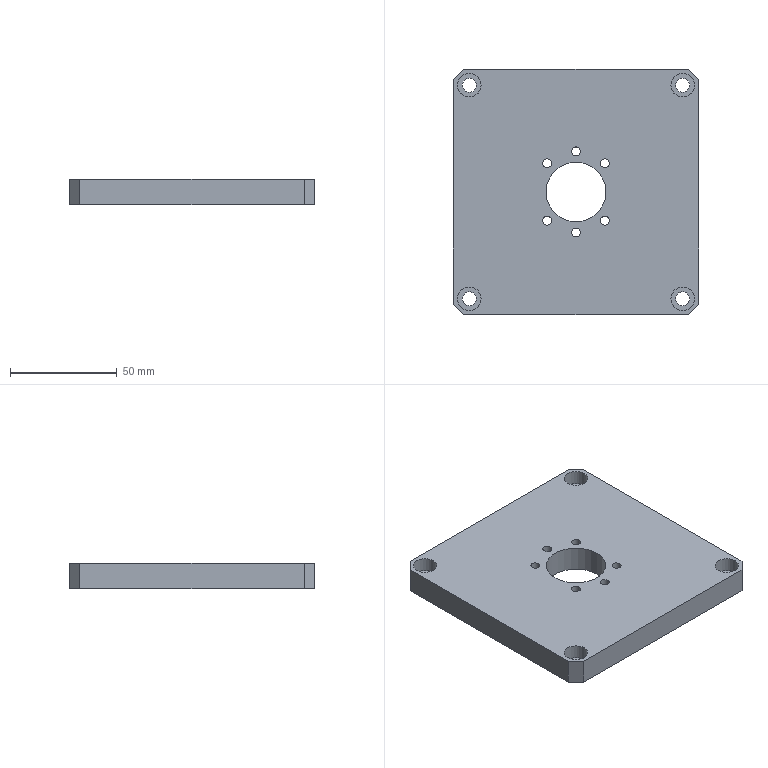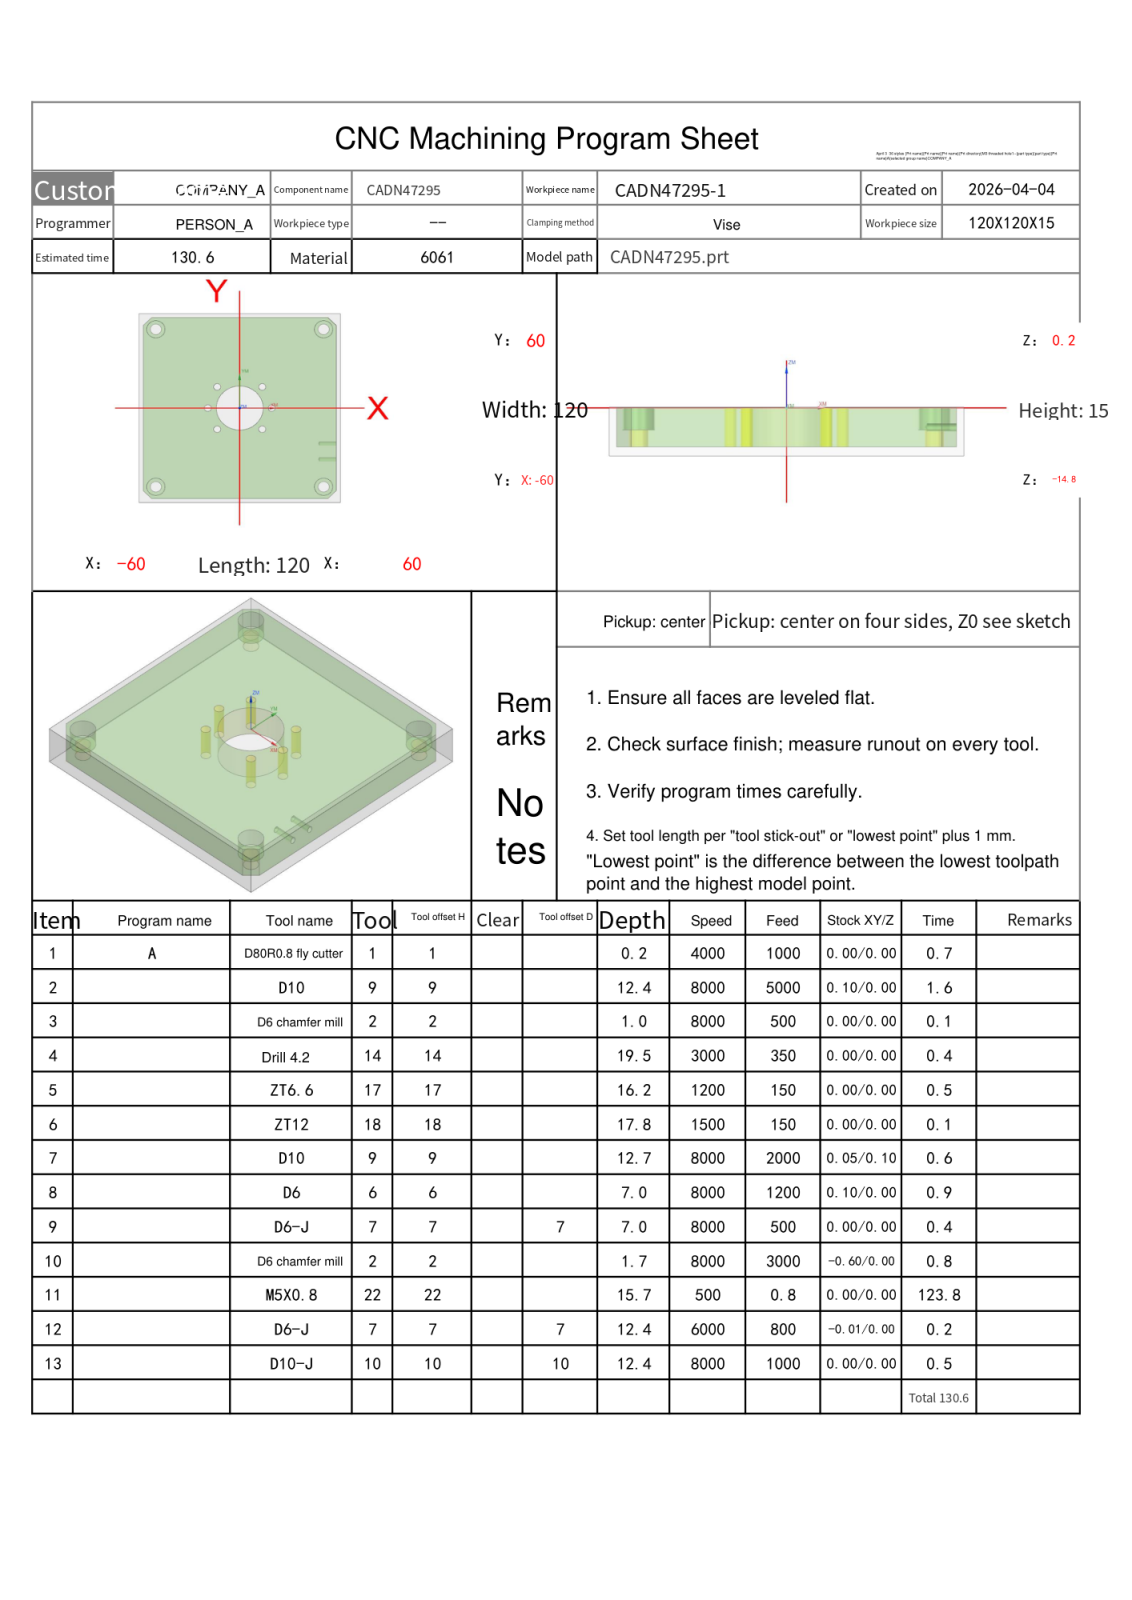NC program | NX | posted by the shop | part box 115 x 115 x 12 mm
Whole program:
%
O0001
(Machine time: 249.39 MIN)
(===Total Tool:10===)
(T1=D80R0.8 fly cutter D=80.  R=0.8  D-  H01 Z=0.    )
(T9=D10     D=10.  R=0.   D-  H09 Z=-12.5 )
(T2=D6 chamfer mill   D=6.   R=0.   D-  H02 Z=-1.5  )
(T14=drill 4.2  D=4.2  DR_a=118 D-  H14 Z=-19.26)
(T17=ZT6.6  D=6.6  DR_a=118 D-  H17 Z=-15.98)
(T18=ZT12   D=12.  DR_a=118 D-  H18 Z=-17.61)
(T6=D6      D=6.   R=0.   D-  H06 Z=-6.8  )
(T7=D6-J    D=6.   R=0.   D7  H07 Z=-12.2 )
(T22=M5X0.8 D=4.2  DR_a=180 D-  H22 Z=-15.5 )
(T10=D10-J  D=10.  R=0.   D10 H10 Z=-12.2 )
G80 G90 G17 G49 G40
G91 G28 Z0
M01
N1 T01 M06
(D80R0.8 fly cutter  D=80. R=0.8 H=01 ce=0.00 di=0.00)
G00 G90 G54 X48.75 Y102.5 M03 S4000
G43 H01 Z20.
M08
Z2.
G01 Z0.0 F1000.
Y97.5
Y-97.5
X0.0
Y97.5
X-48.75
Y-97.5
Y-102.5
Z2.
G00 Z20.
G91 G28 Z0.0
M05
M09
G91 G28 Z0.0
M01
N2 T09 M06
(D10  D=10. R=0. H=09 ce=0.10 di=0.00)
G00 G90 G54 X-62.6 Y0.0 M03 S8000
G43 H09 Z20.
M08
Z.5
G01 Y52.5 Z.413 F5000.
G02 X-61.106 Y56.106 Z.407 I5.1 J0.0
G01 X-56.106 Y61.106 Z.395
G02 X-52.5 Y62.6 Z.388 I3.606 J-3.606
G01 X52.5 Z.215
G02 X56.106 Y61.106 Z.208 I0.0 J-5.1
G01 X61.106 Y56.106 Z.197
G02 X62.6 Y52.5 Z.19 I-3.606 J-3.606
G01 Y-52.5 Z.016
G02 X61.106 Y-56.106 Z.01 I-5.1 J0.0
G01 X56.106 Y-61.106 Z-.002
G02 X52.5 Y-62.6 Z-.009 I-3.606 J3.606
G01 X-52.5 Z-.182
G02 X-56.106 Y-61.106 Z-.189 I0.0 J5.1
G01 X-61.106 Y-56.106 Z-.2
G02 X-62.6 Y-52.5 Z-.207 I3.606 J3.606
G01 Y52.5 Z-.381
G02 X-61.106 Y56.106 Z-.387 I5.1 J0.0
G01 X-56.106 Y61.106 Z-.399
G02 X-52.5 Y62.6 Z-.405 I3.606 J-3.606
G01 X52.5 Z-.579
G02 X56.106 Y61.106 Z-.586 I0.0 J-5.1
G01 X61.106 Y56.106 Z-.597
G02 X62.6 Y52.5 Z-.604 I-3.606 J-3.606
G01 Y-52.5 Z-.777
G02 X61.106 Y-56.106 Z-.784 I-5.1 J0.0
G01 X56.106 Y-61.106 Z-.796
G02 X52.5 Y-62.6 Z-.802 I-3.606 J3.606
G01 X-52.5 Z-.976
G02 X-56.106 Y-61.106 Z-.982 I0.0 J5.1
G01 X-61.106 Y-56.106 Z-.994
G02 X-62.6 Y-52.5 Z-1.001 I3.606 J3.606
G01 Y52.5 Z-1.174
G02 X-61.106 Y56.106 Z-1.181 I5.1 J0.0
G01 X-56.106 Y61.106 Z-1.193
G02 X-52.5 Y62.6 Z-1.199 I3.606 J-3.606
G01 X52.5 Z-1.373
G02 X56.106 Y61.106 Z-1.379 I0.0 J-5.1
G01 X61.106 Y56.106 Z-1.391
G02 X62.6 Y52.5 Z-1.398 I-3.606 J-3.606
G01 Y-52.5 Z-1.571
G02 X61.106 Y-56.106 Z-1.578 I-5.1 J0.0
G01 X56.106 Y-61.106 Z-1.589
G02 X52.5 Y-62.6 Z-1.596 I-3.606 J3.606
G01 X-52.5 Z-1.77
G02 X-56.106 Y-61.106 Z-1.776 I0.0 J5.1
G01 X-61.106 Y-56.106 Z-1.788
G02 X-62.6 Y-52.5 Z-1.794 I3.606 J3.606
G01 Y52.5 Z-1.968
G02 X-61.106 Y56.106 Z-1.975 I5.1 J0.0
G01 X-56.106 Y61.106 Z-1.986
G02 X-52.5 Y62.6 Z-1.993 I3.606 J-3.606
G01 X52.5 Z-2.166
G02 X56.106 Y61.106 Z-2.173 I0.0 J-5.1
G01 X61.106 Y56.106 Z-2.185
G02 X62.6 Y52.5 Z-2.191 I-3.606 J-3.606
G01 Y-52.5 Z-2.365
G02 X61.106 Y-56.106 Z-2.372 I-5.1 J0.0
G01 X56.106 Y-61.106 Z-2.383
G02 X52.5 Y-62.6 Z-2.39 I-3.606 J3.606
G01 X-52.5 Z-2.563
G02 X-56.106 Y-61.106 Z-2.57 I0.0 J5.1
G01 X-61.106 Y-56.106 Z-2.582
G02 X-62.6 Y-52.5 Z-2.588 I3.606 J3.606
G01 Y52.5 Z-2.762
G02 X-61.106 Y56.106 Z-2.768 I5.1 J0.0
G01 X-56.106 Y61.106 Z-2.78
G02 X-52.5 Y62.6 Z-2.787 I3.606 J-3.606
G01 X52.5 Z-2.96
G02 X56.106 Y61.106 Z-2.967 I0.0 J-5.1
G01 X61.106 Y56.106 Z-2.978
G02 X62.6 Y52.5 Z-2.985 I-3.606 J-3.606
G01 Y-52.5 Z-3.159
G02 X61.106 Y-56.106 Z-3.165 I-5.1 J0.0
G01 X56.106 Y-61.106 Z-3.177
G02 X52.5 Y-62.6 Z-3.184 I-3.606 J3.606
G01 X-52.5 Z-3.357
G02 X-56.106 Y-61.106 Z-3.364 I0.0 J5.1
G01 X-61.106 Y-56.106 Z-3.375
G02 X-62.6 Y-52.5 Z-3.382 I3.606 J3.606
G01 Y52.5 Z-3.556
G02 X-61.106 Y56.106 Z-3.562 I5.1 J0.0
G01 X-56.106 Y61.106 Z-3.574
G02 X-52.5 Y62.6 Z-3.58 I3.606 J-3.606
G01 X52.5 Z-3.754
G02 X56.106 Y61.106 Z-3.761 I0.0 J-5.1
G01 X61.106 Y56.106 Z-3.772
G02 X62.6 Y52.5 Z-3.779 I-3.606 J-3.606
G01 Y-52.5 Z-3.952
G02 X61.106 Y-56.106 Z-3.959 I-5.1 J0.0
G01 X56.106 Y-61.106 Z-3.971
G02 X52.5 Y-62.6 Z-3.977 I-3.606 J3.606
G01 X-52.5 Z-4.151
G02 X-56.106 Y-61.106 Z-4.157 I0.0 J5.1
G01 X-61.106 Y-56.106 Z-4.169
G02 X-62.6 Y-52.5 Z-4.176 I3.606 J3.606
G01 Y52.5 Z-4.349
G02 X-61.106 Y56.106 Z-4.356 I5.1 J0.0
G01 X-56.106 Y61.106 Z-4.368
G02 X-52.5 Y62.6 Z-4.374 I3.606 J-3.606
G01 X52.5 Z-4.548
G02 X56.106 Y61.106 Z-4.554 I0.0 J-5.1
G01 X61.106 Y56.106 Z-4.566
G02 X62.6 Y52.5 Z-4.573 I-3.606 J-3.606
G01 Y-52.5 Z-4.746
G02 X61.106 Y-56.106 Z-4.753 I-5.1 J0.0
G01 X56.106 Y-61.106 Z-4.764
G02 X52.5 Y-62.6 Z-4.771 I-3.606 J3.606
G01 X-52.5 Z-4.945
G02 X-56.106 Y-61.106 Z-4.951 I0.0 J5.1
G01 X-61.106 Y-56.106 Z-4.963
G02 X-62.6 Y-52.5 Z-4.969 I3.606 J3.606
G01 Y52.5 Z-5.143
G02 X-61.106 Y56.106 Z-5.15 I5.1 J0.0
G01 X-56.106 Y61.106 Z-5.161
G02 X-52.5 Y62.6 Z-5.168 I3.606 J-3.606
G01 X52.5 Z-5.341
G02 X56.106 Y61.106 Z-5.348 I0.0 J-5.1
G01 X61.106 Y56.106 Z-5.36
G02 X62.6 Y52.5 Z-5.366 I-3.606 J-3.606
G01 Y-52.5 Z-5.54
G02 X61.106 Y-56.106 Z-5.547 I-5.1 J0.0
G01 X56.106 Y-61.106 Z-5.558
G02 X52.5 Y-62.6 Z-5.565 I-3.606 J3.606
G01 X-52.5 Z-5.738
G02 X-56.106 Y-61.106 Z-5.745 I0.0 J5.1
G01 X-61.106 Y-56.106 Z-5.757
G02 X-62.6 Y-52.5 Z-5.763 I3.606 J3.606
G01 Y52.5 Z-5.937
G02 X-61.106 Y56.106 Z-5.943 I5.1 J0.0
G01 X-56.106 Y61.106 Z-5.955
G02 X-52.5 Y62.6 Z-5.962 I3.606 J-3.606
G01 X52.5 Z-6.135
G02 X56.106 Y61.106 Z-6.142 I0.0 J-5.1
G01 X61.106 Y56.106 Z-6.153
G02 X62.6 Y52.5 Z-6.16 I-3.606 J-3.606
G01 Y-52.5 Z-6.334
G02 X61.106 Y-56.106 Z-6.34 I-5.1 J0.0
G01 X56.106 Y-61.106 Z-6.352
G02 X52.5 Y-62.6 Z-6.359 I-3.606 J3.606
G01 X-52.5 Z-6.532
G02 X-56.106 Y-61.106 Z-6.539 I0.0 J5.1
G01 X-61.106 Y-56.106 Z-6.55
G02 X-62.6 Y-52.5 Z-6.557 I3.606 J3.606
G01 Y52.5 Z-6.731
G02 X-61.106 Y56.106 Z-6.737 I5.1 J0.0
G01 X-56.106 Y61.106 Z-6.749
G02 X-52.5 Y62.6 Z-6.755 I3.606 J-3.606
G01 X52.5 Z-6.929
G02 X56.106 Y61.106 Z-6.936 I0.0 J-5.1
G01 X61.106 Y56.106 Z-6.947
G02 X62.6 Y52.5 Z-6.954 I-3.606 J-3.606
G01 Y-52.5 Z-7.127
G02 X61.106 Y-56.106 Z-7.134 I-5.1 J0.0
G01 X56.106 Y-61.106 Z-7.146
G02 X52.5 Y-62.6 Z-7.152 I-3.606 J3.606
G01 X-52.5 Z-7.326
G02 X-56.106 Y-61.106 Z-7.332 I0.0 J5.1
G01 X-61.106 Y-56.106 Z-7.344
G02 X-62.6 Y-52.5 Z-7.351 I3.606 J3.606
G01 Y52.5 Z-7.524
G02 X-61.106 Y56.106 Z-7.531 I5.1 J0.0
G01 X-56.106 Y61.106 Z-7.543
G02 X-52.5 Y62.6 Z-7.549 I3.606 J-3.606
G01 X52.5 Z-7.723
G02 X56.106 Y61.106 Z-7.729 I0.0 J-5.1
G01 X61.106 Y56.106 Z-7.741
G02 X62.6 Y52.5 Z-7.748 I-3.606 J-3.606
G01 Y-52.5 Z-7.921
G02 X61.106 Y-56.106 Z-7.928 I-5.1 J0.0
G01 X56.106 Y-61.106 Z-7.939
G02 X52.5 Y-62.6 Z-7.946 I-3.606 J3.606
G01 X-52.5 Z-8.12
G02 X-56.106 Y-61.106 Z-8.126 I0.0 J5.1
G01 X-61.106 Y-56.106 Z-8.138
G02 X-62.6 Y-52.5 Z-8.144 I3.606 J3.606
G01 Y52.5 Z-8.318
G02 X-61.106 Y56.106 Z-8.325 I5.1 J0.0
G01 X-56.106 Y61.106 Z-8.336
G02 X-52.5 Y62.6 Z-8.343 I3.606 J-3.606
G01 X52.5 Z-8.516
G02 X56.106 Y61.106 Z-8.523 I0.0 J-5.1
G01 X61.106 Y56.106 Z-8.535
G02 X62.6 Y52.5 Z-8.541 I-3.606 J-3.606
G01 Y-52.5 Z-8.715
G02 X61.106 Y-56.106 Z-8.722 I-5.1 J0.0
G01 X56.106 Y-61.106 Z-8.733
G02 X52.5 Y-62.6 Z-8.74 I-3.606 J3.606
G01 X-52.5 Z-8.913
G02 X-56.106 Y-61.106 Z-8.92 I0.0 J5.1
G01 X-61.106 Y-56.106 Z-8.932
G02 X-62.6 Y-52.5 Z-8.938 I3.606 J3.606
G01 Y52.5 Z-9.112
G02 X-61.106 Y56.106 Z-9.118 I5.1 J0.0
G01 X-56.106 Y61.106 Z-9.13
G02 X-52.5 Y62.6 Z-9.137 I3.606 J-3.606
G01 X52.5 Z-9.31
G02 X56.106 Y61.106 Z-9.317 I0.0 J-5.1
G01 X61.106 Y56.106 Z-9.328
G02 X62.6 Y52.5 Z-9.335 I-3.606 J-3.606
G01 Y-52.5 Z-9.509
G02 X61.106 Y-56.106 Z-9.515 I-5.1 J0.0
G01 X56.106 Y-61.106 Z-9.527
G02 X52.5 Y-62.6 Z-9.534 I-3.606 J3.606
G01 X-52.5 Z-9.707
G02 X-56.106 Y-61.106 Z-9.714 I0.0 J5.1
G01 X-61.106 Y-56.106 Z-9.725
G02 X-62.6 Y-52.5 Z-9.732 I3.606 J3.606
G01 Y52.5 Z-9.906
G02 X-61.106 Y56.106 Z-9.912 I5.1 J0.0
G01 X-56.106 Y61.106 Z-9.924
G02 X-52.5 Y62.6 Z-9.93 I3.606 J-3.606
G01 X52.5 Z-10.104
G02 X56.106 Y61.106 Z-10.111 I0.0 J-5.1
G01 X61.106 Y56.106 Z-10.122
G02 X62.6 Y52.5 Z-10.129 I-3.606 J-3.606
G01 Y-52.5 Z-10.302
G02 X61.106 Y-56.106 Z-10.309 I-5.1 J0.0
G01 X56.106 Y-61.106 Z-10.321
G02 X52.5 Y-62.6 Z-10.327 I-3.606 J3.606
G01 X-52.5 Z-10.501
G02 X-56.106 Y-61.106 Z-10.507 I0.0 J5.1
G01 X-61.106 Y-56.106 Z-10.519
G02 X-62.6 Y-52.5 Z-10.526 I3.606 J3.606
G01 Y52.5 Z-10.699
G02 X-61.106 Y56.106 Z-10.706 I5.1 J0.0
G01 X-56.106 Y61.106 Z-10.718
G02 X-52.5 Y62.6 Z-10.724 I3.606 J-3.606
G01 X52.5 Z-10.898
G02 X56.106 Y61.106 Z-10.904 I0.0 J-5.1
G01 X61.106 Y56.106 Z-10.916
G02 X62.6 Y52.5 Z-10.923 I-3.606 J-3.606
G01 Y-52.5 Z-11.096
G02 X61.106 Y-56.106 Z-11.103 I-5.1 J0.0
G01 X56.106 Y-61.106 Z-11.114
G02 X52.5 Y-62.6 Z-11.121 I-3.606 J3.606
G01 X-52.5 Z-11.295
G02 X-56.106 Y-61.106 Z-11.301 I0.0 J5.1
G01 X-61.106 Y-56.106 Z-11.313
G02 X-62.6 Y-52.5 Z-11.319 I3.606 J3.606
G01 Y52.5 Z-11.493
G02 X-61.106 Y56.106 Z-11.5 I5.1 J0.0
G01 X-56.106 Y61.106 Z-11.511
G02 X-52.5 Y62.6 Z-11.518 I3.606 J-3.606
G01 X52.5 Z-11.691
G02 X56.106 Y61.106 Z-11.698 I0.0 J-5.1
G01 X61.106 Y56.106 Z-11.71
G02 X62.6 Y52.5 Z-11.716 I-3.606 J-3.606
G01 Y-52.5 Z-11.89
G02 X61.106 Y-56.106 Z-11.897 I-5.1 J0.0
G01 X56.106 Y-61.106 Z-11.908
G02 X52.5 Y-62.6 Z-11.915 I-3.606 J3.606
G01 X-52.5 Z-12.088
G02 X-56.106 Y-61.106 Z-12.095 I0.0 J5.1
G01 X-61.106 Y-56.106 Z-12.107
G02 X-62.6 Y-52.5 Z-12.113 I3.606 J3.606
G01 Y0.0 Z-12.2
Y52.5
G02 X-61.106 Y56.106 I5.1 J0.0
G01 X-56.106 Y61.106
G02 X-52.5 Y62.6 I3.606 J-3.606
G01 X52.5
G02 X56.106 Y61.106 I0.0 J-5.1
G01 X61.106 Y56.106
G02 X62.6 Y52.5 I-3.606 J-3.606
G01 Y-52.5
G02 X61.106 Y-56.106 I-5.1 J0.0
G01 X56.106 Y-61.106
G02 X52.5 Y-62.6 I-3.606 J3.606
G01 X-52.5
G02 X-56.106 Y-61.106 I0.0 J5.1
G01 X-61.106 Y-56.106
G02 X-62.6 Y-52.5 I3.606 J3.606
G01 Y0.0
Y.5
Z-11.2
G00 Z20.
G91 G28 Z0.0
M05
M09
G91 G28 Z0.0
M01
N3 T02 M06
(D6 chamfer mill  D=6. R=0. H=02 ce=0.00 di=0.00)
G00 G90 G54 X0.0 Y0.0 M03 S8000
G43 H02 Z20.
M08
G98 G82 X0.0 Y0.0 Z-.8 R1. F500.
G80
G00 Z20.
G00 G90 X50. Y50. M03 S8000
Z20.
G98 G81 X50. Y50. Z-.8 R1. F500.
X13.435 Y13.435
X19. Y0.0
X13.435 Y-13.435
X50. Y-50.
X-50.
X-13.435 Y-13.435
X-19. Y0.0
X-13.435 Y13.435
X-50. Y50.
G80
G00 Z20.
G91 G28 Z0.0
M05
M09
G91 G28 Z0.0
M01
N4 T14 M06
(drill 4.2 D=4.2 DR_a=118 H=14)
G00 G90 G54 X-13.435 Y-13.435 M03 S3000
G43 H14 Z20.
M08
G98 G83 X-13.435 Y-13.435 Z-19.262 R1. F350. Q3.
X-19. Y0.0
X-13.435 Y13.435
X13.435
X19. Y0.0
X13.435 Y-13.435
G80
G00 Z20.
G91 G28 Z0.0
M05
M09
G91 G28 Z0.0
M01
N5 T17 M06
(ZT6.6 D=6.6 DR_a=118 H=17)
G00 G90 G54 X-50. Y-50. M03 S1200
G43 H17 Z20.
M08
G98 G83 X-50. Y-50. Z-15.983 R1. F150. Q2.
Y50.
X50.
Y-50.
G80
G00 Z20.
G91 G28 Z0.0
M05
M09
G91 G28 Z0.0
M01
N6 T18 M06
(ZT12 D=12. DR_a=118 H=18)
G00 G90 G54 X0.0 Y0.0 M03 S800
G43 H18 Z20.
M08
G98 G83 X0.0 Y0.0 Z-17.605 R1. F150. Q3.
G80
G00 Z20.
G91 G28 Z0.0
M05
M09
G91 G28 Z0.0
M01
N7 T09 M06
(D10  D=10. R=0. H=09 ce=0.05 di=0.10)
G00 G90 G54 X-7.585 Y4.728 M03 S8000
G43 H09 Z20.
M08
Z1.
G01 X-7.949 Y4.177 Z.965 F2000.
X-8.623 Y2.506 Z.871
X-8.95 Y.733 Z.776
Y-.733 Z.7
X-8.623 Y-2.506 Z.605
X-7.949 Y-4.177 Z.511
X-6.955 Y-5.681 Z.416
X-5.681 Y-6.955 Z.322
X-4.177 Y-7.949 Z.227
X-2.506 Y-8.623 Z.133
X-.733 Y-8.95 Z.038
X0.0 Z0.0
G03 X8.95 Y0.0 Z-.149 I0.0 J8.95
X0.0 Y8.95 Z-.298 I-8.95 J0.0
X-8.95 Y0.0 Z-.446 I0.0 J-8.95
X0.0 Y-8.95 Z-.595 I8.95 J0.0
X8.95 Y0.0 Z-.744 I0.0 J8.95
X0.0 Y8.95 Z-.893 I-8.95 J0.0
X-8.95 Y0.0 Z-1.042 I0.0 J-8.95
X0.0 Y-8.95 Z-1.19 I8.95 J0.0
X8.95 Y0.0 Z-1.339 I0.0 J8.95
X0.0 Y8.95 Z-1.488 I-8.95 J0.0
X-8.95 Y0.0 Z-1.637 I0.0 J-8.95
X0.0 Y-8.95 Z-1.786 I8.95 J0.0
X8.95 Y0.0 Z-1.935 I0.0 J8.95
X0.0 Y8.95 Z-2.083 I-8.95 J0.0
X-8.95 Y0.0 Z-2.232 I0.0 J-8.95
X0.0 Y-8.95 Z-2.381 I8.95 J0.0
X8.95 Y0.0 Z-2.53 I0.0 J8.95
X0.0 Y8.95 Z-2.679 I-8.95 J0.0
X-8.95 Y0.0 Z-2.827 I0.0 J-8.95
X0.0 Y-8.95 Z-2.976 I8.95 J0.0
X8.95 Y0.0 Z-3.125 I0.0 J8.95
X0.0 Y8.95 Z-3.274 I-8.95 J0.0
X-8.95 Y0.0 Z-3.423 I0.0 J-8.95
X0.0 Y-8.95 Z-3.571 I8.95 J0.0
X8.95 Y0.0 Z-3.72 I0.0 J8.95
X0.0 Y8.95 Z-3.869 I-8.95 J0.0
X-8.95 Y0.0 Z-4.018 I0.0 J-8.95
X0.0 Y-8.95 Z-4.167 I8.95 J0.0
X8.95 Y0.0 Z-4.315 I0.0 J8.95
X0.0 Y8.95 Z-4.464 I-8.95 J0.0
X-8.95 Y0.0 Z-4.613 I0.0 J-8.95
X0.0 Y-8.95 Z-4.762 I8.95 J0.0
X8.95 Y0.0 Z-4.911 I0.0 J8.95
X0.0 Y8.95 Z-5.06 I-8.95 J0.0
X-8.95 Y0.0 Z-5.208 I0.0 J-8.95
X0.0 Y-8.95 Z-5.357 I8.95 J0.0
X8.95 Y0.0 Z-5.506 I0.0 J8.95
X0.0 Y8.95 Z-5.655 I-8.95 J0.0
X-8.95 Y0.0 Z-5.804 I0.0 J-8.95
X0.0 Y-8.95 Z-5.952 I8.95 J0.0
X8.95 Y0.0 Z-6.101 I0.0 J8.95
X0.0 Y8.95 Z-6.25 I-8.95 J0.0
X-8.95 Y0.0 Z-6.399 I0.0 J-8.95
X0.0 Y-8.95 Z-6.548 I8.95 J0.0
X8.95 Y0.0 Z-6.696 I0.0 J8.95
X0.0 Y8.95 Z-6.845 I-8.95 J0.0
X-8.95 Y0.0 Z-6.994 I0.0 J-8.95
X0.0 Y-8.95 Z-7.143 I8.95 J0.0
X8.95 Y0.0 Z-7.292 I0.0 J8.95
X0.0 Y8.95 Z-7.44 I-8.95 J0.0
X-8.95 Y0.0 Z-7.589 I0.0 J-8.95
X0.0 Y-8.95 Z-7.738 I8.95 J0.0
X8.95 Y0.0 Z-7.887 I0.0 J8.95
X0.0 Y8.95 Z-8.036 I-8.95 J0.0
X-8.95 Y0.0 Z-8.185 I0.0 J-8.95
X0.0 Y-8.95 Z-8.333 I8.95 J0.0
X8.95 Y0.0 Z-8.482 I0.0 J8.95
X0.0 Y8.95 Z-8.631 I-8.95 J0.0
X-8.95 Y0.0 Z-8.78 I0.0 J-8.95
X0.0 Y-8.95 Z-8.929 I8.95 J0.0
X8.95 Y0.0 Z-9.077 I0.0 J8.95
X0.0 Y8.95 Z-9.226 I-8.95 J0.0
X-8.95 Y0.0 Z-9.375 I0.0 J-8.95
X0.0 Y-8.95 Z-9.524 I8.95 J0.0
X8.95 Y0.0 Z-9.673 I0.0 J8.95
X0.0 Y8.95 Z-9.821 I-8.95 J0.0
X-8.95 Y0.0 Z-9.97 I0.0 J-8.95
X0.0 Y-8.95 Z-10.119 I8.95 J0.0
X8.95 Y0.0 Z-10.268 I0.0 J8.95
X0.0 Y8.95 Z-10.417 I-8.95 J0.0
X-8.95 Y0.0 Z-10.565 I0.0 J-8.95
X0.0 Y-8.95 Z-10.714 I8.95 J0.0
X8.95 Y0.0 Z-10.863 I0.0 J8.95
X0.0 Y8.95 Z-11.012 I-8.95 J0.0
X-8.95 Y0.0 Z-11.161 I0.0 J-8.95
X0.0 Y-8.95 Z-11.31 I8.95 J0.0
X8.95 Y0.0 Z-11.458 I0.0 J8.95
X0.0 Y8.95 Z-11.607 I-8.95 J0.0
X-8.95 Y0.0 Z-11.756 I0.0 J-8.95
X0.0 Y-8.95 Z-11.905 I8.95 J0.0
X8.95 Y0.0 Z-12.054 I0.0 J8.95
X0.0 Y8.95 Z-12.202 I-8.95 J0.0
X-8.95 Y0.0 Z-12.351 I0.0 J-8.95
X0.0 Y-8.95 Z-12.5 I8.95 J0.0
X8.95 Y0.0 I0.0 J8.95
X0.0 Y8.95 I-8.95 J0.0
X-8.95 Y0.0 I0.0 J-8.95
X0.0 Y-8.95 I8.95 J0.0
X.4 Y-8.941 I0.0 J8.95
G01 Z-11.5
G00 Z20.
G91 G28 Z0.0
M05
M09
G91 G28 Z0.0
M01
N8 T06 M06
(D6  D=6. R=0. H=06 ce=0.10 di=0.00)
G00 G90 G54 X-50. Y-50. M03 S8000
G43 H06 Z20.
M08
Z.5
G03 X-51.2 Y-51.2 I0.0 J-1.2 F1200.
X-50. Y-52.4 I1.2 J0.0
X-50. Y-52.4 Z0.0 I0.0 J2.4
X-50. Y-52.4 Z-.5 I0.0 J2.4
X-50. Y-52.4 Z-1. I0.0 J2.4
X-50. Y-52.4 Z-1.5 I0.0 J2.4
X-50. Y-52.4 Z-2. I0.0 J2.4
X-50. Y-52.4 Z-2.5 I0.0 J2.4
X-50. Y-52.4 Z-3. I0.0 J2.4
X-50. Y-52.4 Z-3.5 I0.0 J2.4
X-50. Y-52.4 Z-4. I0.0 J2.4
X-50. Y-52.4 Z-4.5 I0.0 J2.4
X-50. Y-52.4 Z-5. I0.0 J2.4
X-50. Y-52.4 Z-5.5 I0.0 J2.4
X-50. Y-52.4 Z-6. I0.0 J2.4
X-50. Y-52.4 Z-6.5 I0.0 J2.4
X-51.411 Y-48.058 Z-6.8 I0.0 J2.4
X-52.4 Y-50. I1.411 J-1.942
X-50. Y-52.4 I2.4 J0.0
X-47.6 Y-50. I0.0 J2.4
X-50. Y-47.6 I-2.4 J0.0
X-51.411 Y-48.058 I0.0 J-2.4
X-51.905 Y-49.029 I.705 J-.971
X-50.705 Y-50.229 I1.2 J0.0
X-50. Y-50. I0.0 J1.2
G00 Z20.
Y50.
Z.5
G03 X-51.2 Y48.8 I0.0 J-1.2
X-50. Y47.6 I1.2 J0.0
X-50. Y47.6 Z0.0 I0.0 J2.4
X-50. Y47.6 Z-.5 I0.0 J2.4
X-50. Y47.6 Z-1. I0.0 J2.4
X-50. Y47.6 Z-1.5 I0.0 J2.4
X-50. Y47.6 Z-2. I0.0 J2.4
X-50. Y47.6 Z-2.5 I0.0 J2.4
X-50. Y47.6 Z-3. I0.0 J2.4
X-50. Y47.6 Z-3.5 I0.0 J2.4
X-50. Y47.6 Z-4. I0.0 J2.4
X-50. Y47.6 Z-4.5 I0.0 J2.4
X-50. Y47.6 Z-5. I0.0 J2.4
X-50. Y47.6 Z-5.5 I0.0 J2.4
X-50. Y47.6 Z-6. I0.0 J2.4
X-50. Y47.6 Z-6.5 I0.0 J2.4
X-51.411 Y51.942 Z-6.8 I0.0 J2.4
X-52.4 Y50. I1.411 J-1.942
X-50. Y47.6 I2.4 J0.0
X-47.6 Y50. I0.0 J2.4
X-50. Y52.4 I-2.4 J0.0
X-51.411 Y51.942 I0.0 J-2.4
X-51.905 Y50.971 I.705 J-.971
X-50.705 Y49.771 I1.2 J0.0
X-50. Y50. I0.0 J1.2
G00 Z20.
X50.
Z.5
G03 X48.8 Y48.8 I0.0 J-1.2
X50. Y47.6 I1.2 J0.0
X50. Y47.6 Z0.0 I0.0 J2.4
X50. Y47.6 Z-.5 I0.0 J2.4
X50. Y47.6 Z-1. I0.0 J2.4
X50. Y47.6 Z-1.5 I0.0 J2.4
X50. Y47.6 Z-2. I0.0 J2.4
X50. Y47.6 Z-2.5 I0.0 J2.4
X50. Y47.6 Z-3. I0.0 J2.4
X50. Y47.6 Z-3.5 I0.0 J2.4
X50. Y47.6 Z-4. I0.0 J2.4
X50. Y47.6 Z-4.5 I0.0 J2.4
X50. Y47.6 Z-5. I0.0 J2.4
X50. Y47.6 Z-5.5 I0.0 J2.4
X50. Y47.6 Z-6. I0.0 J2.4
X50. Y47.6 Z-6.5 I0.0 J2.4
X48.589 Y51.942 Z-6.8 I0.0 J2.4
X47.6 Y50. I1.411 J-1.942
X50. Y47.6 I2.4 J0.0
X52.4 Y50. I0.0 J2.4
X50. Y52.4 I-2.4 J0.0
X48.589 Y51.942 I0.0 J-2.4
X48.095 Y50.971 I.705 J-.971
X49.295 Y49.771 I1.2 J0.0
X50. Y50. I0.0 J1.2
G00 Z20.
Y-50.
Z.5
G03 X48.8 Y-51.2 I0.0 J-1.2
X50. Y-52.4 I1.2 J0.0
X50. Y-52.4 Z0.0 I0.0 J2.4
X50. Y-52.4 Z-.5 I0.0 J2.4
X50. Y-52.4 Z-1. I0.0 J2.4
X50. Y-52.4 Z-1.5 I0.0 J2.4
X50. Y-52.4 Z-2. I0.0 J2.4
X50. Y-52.4 Z-2.5 I0.0 J2.4
X50. Y-52.4 Z-3. I0.0 J2.4
X50. Y-52.4 Z-3.5 I0.0 J2.4
X50. Y-52.4 Z-4. I0.0 J2.4
X50. Y-52.4 Z-4.5 I0.0 J2.4
X50. Y-52.4 Z-5. I0.0 J2.4
X50. Y-52.4 Z-5.5 I0.0 J2.4
X50. Y-52.4 Z-6. I0.0 J2.4
X50. Y-52.4 Z-6.5 I0.0 J2.4
X48.589 Y-48.058 Z-6.8 I0.0 J2.4
X47.6 Y-50. I1.411 J-1.942
X50. Y-52.4 I2.4 J0.0
X52.4 Y-50. I0.0 J2.4
X50. Y-47.6 I-2.4 J0.0
X48.589 Y-48.058 I0.0 J-2.4
X48.095 Y-49.029 I.705 J-.971
X49.295 Y-50.229 I1.2 J0.0
X50. Y-50. I0.0 J1.2
G00 Z20.
G91 G28 Z0.0
M05
M09
G91 G28 Z0.0
M01
N9 T07 M06
(D6-J  D=6. R=0. H=07 ce=0.00 di=0.00)
G00 G90 G54 X-50. Y-50. M03 S8000
G43 H07 Z20.
M08
Z0.0
G41 D07
G01 X-50.197 Y-50.032 F500.
G03 X-51.242 Y-51.258 I.197 J-1.226
X-50. Y-52.5 I1.242 J0.0
X-50. Y-52.5 Z-5. I0.0 J2.5
X-48.074 Y-48.406 Z-6.8 I0.0 J2.5
X-50. Y-47.5 I-1.926 J-1.594
X-52.5 Y-50. I0.0 J-2.5
X-50. Y-52.5 I2.5 J0.0
X-47.5 Y-50. I0.0 J2.5
X-48.074 Y-48.406 I-2.5 J0.0
X-49.031 Y-47.956 I-.957 J-.792
X-50.273 Y-49.198 I0.0 J-1.242
X-50.101 Y-49.828 I1.242 J0.0
G01 G40 X-50. Y-50.
G00 Z20.
Y50.
Z0.0
G41 D07
G01 X-50.197 Y49.968
G03 X-51.242 Y48.742 I.197 J-1.226
X-50. Y47.5 I1.242 J0.0
X-50. Y47.5 Z-5. I0.0 J2.5
X-48.074 Y51.594 Z-6.8 I0.0 J2.5
X-50. Y52.5 I-1.926 J-1.594
X-52.5 Y50. I0.0 J-2.5
X-50. Y47.5 I2.5 J0.0
X-47.5 Y50. I0.0 J2.5
X-48.074 Y51.594 I-2.5 J0.0
X-49.031 Y52.044 I-.957 J-.792
X-50.273 Y50.802 I0.0 J-1.242
X-50.101 Y50.172 I1.242 J0.0
G01 G40 X-50. Y50.
G00 Z20.
X50.
Z0.0
G41 D07
G01 X49.803 Y49.968
G03 X48.758 Y48.742 I.197 J-1.226
X50. Y47.5 I1.242 J0.0
X50. Y47.5 Z-5. I0.0 J2.5
X51.926 Y51.594 Z-6.8 I0.0 J2.5
X50. Y52.5 I-1.926 J-1.594
X47.5 Y50. I0.0 J-2.5
X50. Y47.5 I2.5 J0.0
X52.5 Y50. I0.0 J2.5
X51.926 Y51.594 I-2.5 J0.0
X50.969 Y52.044 I-.957 J-.792
X49.727 Y50.802 I0.0 J-1.242
X49.899 Y50.172 I1.242 J0.0
G01 G40 X50. Y50.
G00 Z20.
Y-50.
Z0.0
G41 D07
G01 X49.803 Y-50.032
G03 X48.758 Y-51.258 I.197 J-1.226
X50. Y-52.5 I1.242 J0.0
X50. Y-52.5 Z-5. I0.0 J2.5
X51.926 Y-48.406 Z-6.8 I0.0 J2.5
X50. Y-47.5 I-1.926 J-1.594
X47.5 Y-50. I0.0 J-2.5
X50. Y-52.5 I2.5 J0.0
X52.5 Y-50. I0.0 J2.5
X51.926 Y-48.406 I-2.5 J0.0
X50.969 Y-47.956 I-.957 J-.792
X49.727 Y-49.198 I0.0 J-1.242
X49.899 Y-49.828 I1.242 J0.0
G01 G40 X50. Y-50.
G00 Z20.
G91 G28 Z0.0
M05
M09
G91 G28 Z0.0
M01
N10 T02 M06
(D6 chamfer mill  D=6. R=0. H=02 ce=0.00 di=0.00)
G00 G90 G54 X.25 Y-59.628 M03 S8000
G43 H02 Z20.
M08
Z2.099
G01 Z-1.5 F3000.
G03 X.33 Y-59.328 I-.52 J.3
X.03 Y-58.808 I-.6 J0.0
G01 X0.0 Y-58.8
X-52.5
X-52.754 Y-58.775
X-52.997 Y-58.701
X-53.222 Y-58.581
X-53.419 Y-58.419
X-58.419 Y-53.419
X-58.581 Y-53.222
X-58.701 Y-52.997
X-58.775 Y-52.754
X-58.8 Y-52.5
Y52.5
X-58.775 Y52.754
X-58.701 Y52.997
X-58.581 Y53.222
X-58.419 Y53.419
X-53.419 Y58.419
X-53.222 Y58.581
X-52.997 Y58.701
X-52.754 Y58.775
X-52.5 Y58.8
X52.5
X52.754 Y58.775
X52.997 Y58.701
X53.222 Y58.581
X53.419 Y58.419
X58.419 Y53.419
X58.581 Y53.222
X58.701 Y52.997
X58.775 Y52.754
X58.8 Y52.5
Y-52.5
X58.775 Y-52.754
X58.701 Y-52.997
X58.581 Y-53.222
X58.419 Y-53.419
X53.419 Y-58.419
X53.222 Y-58.581
X52.997 Y-58.701
X52.754 Y-58.775
X52.5 Y-58.8
X0.0
X-.03 Y-58.808
G03 X-.33 Y-59.328 I.3 J-.52
X-.25 Y-59.628 I.6 J0.0
G01 Z2.099
G00 Z20.
X.28 Y11.882
Z2.121
G01 Z-1.5
G03 X.35 Y12.163 I-.53 J.28
X.03 Y12.693 I-.6 J0.0
G01 X0.0 Y12.7
G03 X-12.7 Y0.0 I0.0 J-12.7
X0.0 Y-12.7 I12.7 J0.0
X12.7 Y0.0 I0.0 J12.7
X0.0 Y12.7 I-12.7 J0.0
G01 X-.03 Y12.693
G03 X-.35 Y12.163 I.28 J-.53
X-.28 Y11.882 I.6 J0.0
G01 Z2.121
G00 Z20.
G00 G90 X-12.741 Y13.528 M03 S8000
Z20.
Z-.5
G01 Z-1. F500.
X-11.935 Y13.635
G03 X-13.435 Y15.135 I-1.5 J0.0
X-15.135 Y13.435 I0.0 J-1.7
X-13.435 Y11.735 I1.7 J0.0
X-11.735 Y13.435 I0.0 J1.7
X-13.435 Y15.135 I-1.7 J0.0
X-14.935 Y13.635 I0.0 J-1.5
G01 X-14.129 Y13.528
Z-.5
G00 Z20.
X-18.306 Y.093
Z-.5
G01 Z-1.
X-17.5 Y.2
G03 X-19. Y1.7 I-1.5 J0.0
X-20.7 Y0.0 I0.0 J-1.7
X-19. Y-1.7 I1.7 J0.0
X-17.3 Y0.0 I0.0 J1.7
X-19. Y1.7 I-1.7 J0.0
X-20.5 Y.2 I0.0 J-1.5
G01 X-19.694 Y.093
Z-.5
G00 Z20.
X-12.741 Y-13.343
Z-.5
G01 Z-1.
X-11.935 Y-13.235
G03 X-13.435 Y-11.735 I-1.5 J0.0
X-15.135 Y-13.435 I0.0 J-1.7
X-13.435 Y-15.135 I1.7 J0.0
X-11.735 Y-13.435 I0.0 J1.7
X-13.435 Y-11.735 I-1.7 J0.0
X-14.935 Y-13.235 I0.0 J-1.5
G01 X-14.129 Y-13.343
Z-.5
G00 Z20.
X14.129
Z-.5
G01 Z-1.
X14.935 Y-13.235
G03 X13.435 Y-11.735 I-1.5 J0.0
X11.735 Y-13.435 I0.0 J-1.7
X13.435 Y-15.135 I1.7 J0.0
X15.135 Y-13.435 I0.0 J1.7
X13.435 Y-11.735 I-1.7 J0.0
X11.935 Y-13.235 I0.0 J-1.5
G01 X12.741 Y-13.343
Z-.5
G00 Z20.
X19.694 Y.093
Z-.5
G01 Z-1.
X20.5 Y.2
G03 X19. Y1.7 I-1.5 J0.0
X17.3 Y0.0 I0.0 J-1.7
X19. Y-1.7 I1.7 J0.0
X20.7 Y0.0 I0.0 J1.7
X19. Y1.7 I-1.7 J0.0
X17.5 Y.2 I0.0 J-1.5
G01 X18.306 Y.093
Z-.5
G00 Z20.
X14.129 Y13.528
Z-.5
G01 Z-1.
X14.935 Y13.635
G03 X13.435 Y15.135 I-1.5 J0.0
X11.735 Y13.435 I0.0 J-1.7
X13.435 Y11.735 I1.7 J0.0
X15.135 Y13.435 I0.0 J1.7
X13.435 Y15.135 I-1.7 J0.0
X11.935 Y13.635 I0.0 J-1.5
G01 X12.741 Y13.528
Z-.5
G00 Z20.
G00 G90 X45.643 Y52.009 M03 S8000
Z20.
Z2.5
G01 X45.561 Y51.834 Z2.43 F800.
X45.405 Y51.399 Z2.261
X45.292 Y50.95 Z2.093
X45.222 Y50.493 Z1.925
X45.197 Y50.031 Z1.756
X45.216 Y49.569 Z1.588
X45.28 Y49.11 Z1.419
X45.388 Y48.66 Z1.251
X45.538 Y48.223 Z1.083
X45.73 Y47.802 Z.914
X45.961 Y47.401 Z.746
X46.23 Y47.024 Z.577
X46.534 Y46.675 Z.409
X46.87 Y46.357 Z.241
X47.235 Y46.073 Z.072
X47.625 Y45.825 Z-.096
X48.038 Y45.616 Z-.265
X48.469 Y45.448 Z-.433
X48.914 Y45.321 Z-.601
X49.369 Y45.239 Z-.77
X49.83 Y45.2 Z-.938
X50. Z-1.
G03 X54.8 Y50. I0.0 J4.8
X50. Y54.8 I-4.8 J0.0
X45.2 Y50. I0.0 J-4.8
X50. Y45.2 I4.8 J0.0
X50.499 Y45.226 I0.0 J4.8
G01 Z1.5
G00 Z20.
X-54.357 Y52.009
Z2.5
G01 X-54.439 Y51.834 Z2.43
X-54.595 Y51.399 Z2.261
X-54.708 Y50.95 Z2.093
X-54.778 Y50.493 Z1.925
X-54.803 Y50.031 Z1.756
X-54.784 Y49.569 Z1.588
X-54.72 Y49.11 Z1.419
X-54.612 Y48.66 Z1.251
X-54.462 Y48.223 Z1.083
X-54.27 Y47.802 Z.914
X-54.039 Y47.401 Z.746
X-53.77 Y47.024 Z.577
X-53.466 Y46.675 Z.409
X-53.13 Y46.357 Z.241
X-52.765 Y46.073 Z.072
X-52.375 Y45.825 Z-.096
X-51.962 Y45.616 Z-.265
X-51.531 Y45.448 Z-.433
X-51.086 Y45.321 Z-.601
X-50.631 Y45.239 Z-.77
X-50.17 Y45.2 Z-.938
X-50. Z-1.
G03 X-45.2 Y50. I0.0 J4.8
X-50. Y54.8 I-4.8 J0.0
X-54.8 Y50. I0.0 J-4.8
X-50. Y45.2 I4.8 J0.0
X-49.501 Y45.226 I0.0 J4.8
G01 Z1.5
G00 Z20.
X-54.357 Y-47.991
Z2.5
G01 X-54.439 Y-48.166 Z2.43
X-54.595 Y-48.601 Z2.261
X-54.708 Y-49.05 Z2.093
X-54.778 Y-49.507 Z1.925
X-54.803 Y-49.969 Z1.756
X-54.784 Y-50.431 Z1.588
X-54.72 Y-50.89 Z1.419
X-54.612 Y-51.34 Z1.251
X-54.462 Y-51.777 Z1.083
X-54.27 Y-52.198 Z.914
X-54.039 Y-52.599 Z.746
X-53.77 Y-52.976 Z.577
X-53.466 Y-53.325 Z.409
X-53.13 Y-53.643 Z.241
X-52.765 Y-53.927 Z.072
X-52.375 Y-54.175 Z-.096
X-51.962 Y-54.384 Z-.265
X-51.531 Y-54.552 Z-.433
X-51.086 Y-54.679 Z-.601
X-50.631 Y-54.761 Z-.77
X-50.17 Y-54.8 Z-.938
X-50. Z-1.
G03 X-45.2 Y-50. I0.0 J4.8
X-50. Y-45.2 I-4.8 J0.0
X-54.8 Y-50. I0.0 J-4.8
X-50. Y-54.8 I4.8 J0.0
X-49.501 Y-54.774 I0.0 J4.8
G01 Z1.5
G00 Z20.
X45.643 Y-47.991
Z2.5
G01 X45.561 Y-48.166 Z2.43
X45.405 Y-48.601 Z2.261
X45.292 Y-49.05 Z2.093
X45.222 Y-49.507 Z1.925
X45.197 Y-49.969 Z1.756
X45.216 Y-50.431 Z1.588
X45.28 Y-50.89 Z1.419
X45.388 Y-51.34 Z1.251
X45.538 Y-51.777 Z1.083
X45.73 Y-52.198 Z.914
X45.961 Y-52.599 Z.746
X46.23 Y-52.976 Z.577
X46.534 Y-53.325 Z.409
X46.87 Y-53.643 Z.241
X47.235 Y-53.927 Z.072
X47.625 Y-54.175 Z-.096
X48.038 Y-54.384 Z-.265
X48.469 Y-54.552 Z-.433
X48.914 Y-54.679 Z-.601
X49.369 Y-54.761 Z-.77
X49.83 Y-54.8 Z-.938
X50. Z-1.
G03 X54.8 Y-50. I0.0 J4.8
X50. Y-45.2 I-4.8 J0.0
X45.2 Y-50. I0.0 J-4.8
X50. Y-54.8 I4.8 J0.0
X50.499 Y-54.774 I0.0 J4.8
G01 Z1.5
G00 Z20.
G00 G90 X3. Y10.3 M03 S8000
Z20.
Z-.5
G01 Z-1. F800.
G03 X0.0 Y13.3 I-3. J0.0
X-13.3 Y0.0 I0.0 J-13.3
X0.0 Y-13.3 I13.3 J0.0
X13.3 Y0.0 I0.0 J13.3
X0.0 Y13.3 I-13.3 J0.0
X-3. Y10.3 I0.0 J-3.
G01 Z-.5
G00 Z20.
G91 G28 Z0.0
M05
M09
G91 G28 Z0.0
M01
N11 T22 M06
(M5X0.8 D=4.2 DR_a=180 H=22)
G00 G90 G54 X-13.435 Y-13.435 M03 S500
G43 H22 Z20.
M08
G95
G98 G84 X-13.435 Y-13.435 Z-15.5 R1. F.8 Q3.
X-19. Y0.0
X-13.435 Y13.435
X13.435
X19. Y0.0
X13.435 Y-13.435
G80
G94
G00 Z20.
G91 G28 Z0.0
M05
M09
G91 G28 Z0.0
M01
N12 T07 M06
(D6-J  D=6. R=0. H=07 ce=-0.01 di=0.00)
G00 G90 G54 X.9 Y9.875 M03 S6000
G43 H07 Z10.2
M08
Z-4.6
G01 Z-6.1 F800.
G41 D07
Y10.115
G03 X0.0 Y11.015 I-.9 J0.0
X-11.015 Y0.0 I0.0 J-11.015
X0.0 Y-11.015 I11.015 J0.0
X11.015 Y0.0 I0.0 J11.015
X0.0 Y11.015 I-11.015 J0.0
X-.4 Y11.008 I0.0 J-11.015
X-1.267 Y10.108 I.033 J-.899
G01 Y10.076
X-1.265 Y10.036
G40 X-1.258 Y9.836
Z-4.6
G00 X.9 Y9.875
Z-10.7
G01 Z-12.2
G41 D07
Y10.115
G03 X0.0 Y11.015 I-.9 J0.0
X-11.015 Y0.0 I0.0 J-11.015
X0.0 Y-11.015 I11.015 J0.0
X11.015 Y0.0 I0.0 J11.015
X0.0 Y11.015 I-11.015 J0.0
X-.4 Y11.008 I0.0 J-11.015
X-1.267 Y10.108 I.033 J-.899
G01 Y10.076
X-1.265 Y10.036
G40 X-1.258 Y9.836
Z-10.7
G00 Z10.2
G91 G28 Z0.0
M05
M09
G91 G28 Z0.0
M01
N13 T10 M06
(D10-J  D=10. R=0. H=10 ce=0.00 di=0.00)
G00 G90 G54 X-63.616 Y-53.513 M03 S8000
G43 H10 Z20.
M08
Z-11.7
G01 Z-12.2 F1000.
G41 D10
X-63.417 Y-53.497
G03 X-62.5 Y-52.5 I-.083 J.997
G01 Y52.5
G02 X-61.036 Y56.036 I5. J0.0
G01 X-56.036 Y61.036
G02 X-52.5 Y62.5 I3.536 J-3.536
G01 X52.5
G02 X56.036 Y61.036 I0.0 J-5.
G01 X61.036 Y56.036
G02 X62.5 Y52.5 I-3.536 J-3.536
G01 Y-52.5
G02 X61.036 Y-56.036 I-5. J0.0
G01 X56.036 Y-61.036
G02 X52.5 Y-62.5 I-3.536 J3.536
G01 X-52.5
G02 X-56.036 Y-61.036 I0.0 J5.
G01 X-61.036 Y-56.036
G02 X-62.5 Y-52.5 I3.536 J3.536
G01 Y-52.
G03 X-63.5 Y-51. I-1. J0.0
G01 G40 X-63.7
Z-11.7
G00 Z20.
M05
M09
G91 G28 Z0.0
G91 G28 Y0.0
M30
%